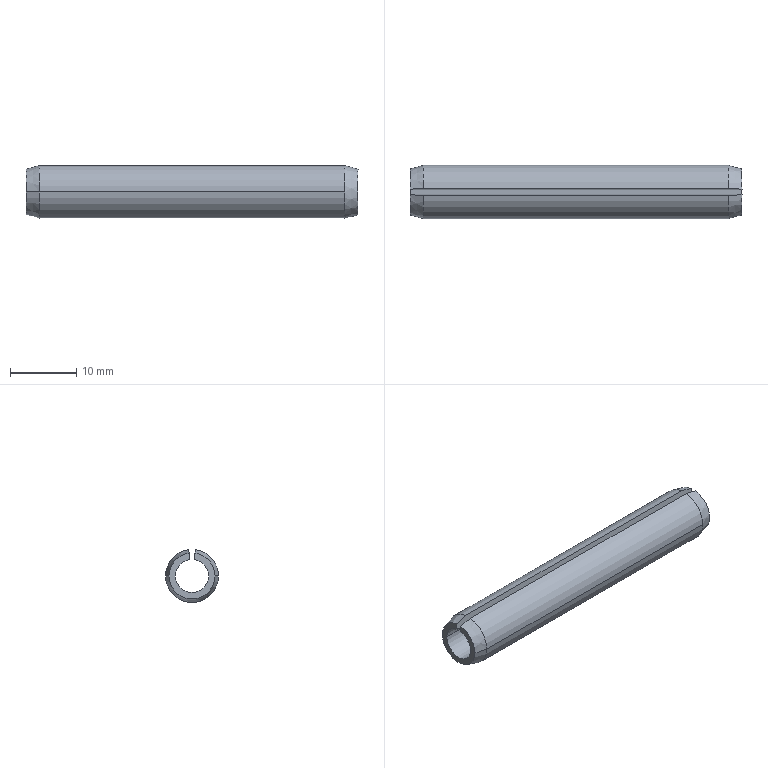Part | SolidWorks | features BaseBody 1 | 1 solid | 14 faces | box 50 x 8 x 7.968 mm | volume 1446 mm3 | cylinder 6 | cone 4 | plane 4 | commonest cylinder face diameters 5 x3 8 x3